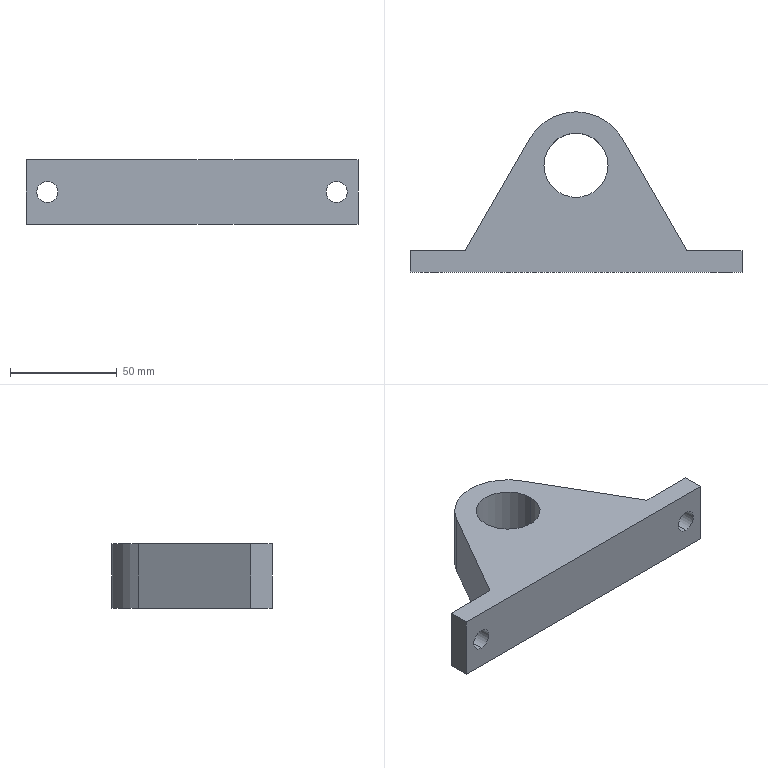Part | SolidWorks | features BaseBody 1 | 1 solid | 18 faces | box 155.5 x 75 x 30 mm | volume 151396 mm3 | plane 10 | cylinder 8 | commonest cylinder face diameters 10 x4 30 x2 50.026 x2
STEP:
#1=CARTESIAN_POINT('',(-375.282,7.138,-265.));
#2=VERTEX_POINT('',#1);
#3=CARTESIAN_POINT('',(-375.282,7.138,-275.));
#4=VERTEX_POINT('',#3);
#5=CARTESIAN_POINT('',(-375.282,7.138,-270.));
#6=DIRECTION('',(0.,-1.,0.));
#7=DIRECTION('',(0.,0.,1.));
#8=AXIS2_PLACEMENT_3D('',#5,#6,#7);
#9=CIRCLE('',#8,5.);
#10=EDGE_CURVE('',#2,#4,#9,.T.);
#11=ORIENTED_EDGE('',*,*,#10,.T.);
#12=CARTESIAN_POINT('',(-375.282,17.138,-275.));
#13=VERTEX_POINT('',#12);
#14=CARTESIAN_POINT('',(-375.282,-2.862,-275.));
#15=DIRECTION('',(0.,1.,0.));
#16=VECTOR('',#15,1000.);
#17=LINE('',#14,#16);
#18=EDGE_CURVE('',#4,#13,#17,.T.);
#19=ORIENTED_EDGE('',*,*,#18,.T.);
#20=CARTESIAN_POINT('',(-375.282,17.138,-265.));
#21=VERTEX_POINT('',#20);
#22=CARTESIAN_POINT('',(-375.282,17.138,-270.));
#23=DIRECTION('',(0.,1.,0.));
#24=DIRECTION('',(0.,0.,1.));
#25=AXIS2_PLACEMENT_3D('',#22,#23,#24);
#26=CIRCLE('',#25,5.);
#27=EDGE_CURVE('',#13,#21,#26,.T.);
#28=ORIENTED_EDGE('',*,*,#27,.T.);
#29=CARTESIAN_POINT('',(-375.282,-2.862,-265.));
#30=DIRECTION('',(0.,1.,0.));
#31=VECTOR('',#30,1000.);
#32=LINE('',#29,#31);
#33=EDGE_CURVE('',#2,#21,#32,.T.);
#34=ORIENTED_EDGE('',*,*,#33,.F.);
#35=EDGE_LOOP('',(#11,#19,#28,#34));
#36=FACE_OUTER_BOUND('',#35,.T.);
#37=CARTESIAN_POINT('',(-375.282,-2.862,-270.));
#38=DIRECTION('',(0.,1.,0.));
#39=DIRECTION('',(0.,0.,1.));
#40=AXIS2_PLACEMENT_3D('',#37,#38,#39);
#41=CYLINDRICAL_SURFACE('',#40,5.);
#42=ADVANCED_FACE('',(#36),#41,.F.);
#43=CARTESIAN_POINT('',(-510.782,7.138,-265.));
#44=VERTEX_POINT('',#43);
#45=CARTESIAN_POINT('',(-510.782,7.138,-275.));
#46=VERTEX_POINT('',#45);
#47=CARTESIAN_POINT('',(-510.782,7.138,-270.));
#48=DIRECTION('',(0.,-1.,0.));
#49=DIRECTION('',(0.,0.,1.));
#50=AXIS2_PLACEMENT_3D('',#47,#48,#49);
#51=CIRCLE('',#50,5.);
#52=EDGE_CURVE('',#44,#46,#51,.T.);
#53=ORIENTED_EDGE('',*,*,#52,.T.);
#54=CARTESIAN_POINT('',(-510.782,17.138,-275.));
#55=VERTEX_POINT('',#54);
#56=CARTESIAN_POINT('',(-510.782,-2.862,-275.));
#57=DIRECTION('',(0.,1.,0.));
#58=VECTOR('',#57,1000.);
#59=LINE('',#56,#58);
#60=EDGE_CURVE('',#46,#55,#59,.T.);
#61=ORIENTED_EDGE('',*,*,#60,.T.);
#62=CARTESIAN_POINT('',(-510.782,17.138,-265.));
#63=VERTEX_POINT('',#62);
#64=CARTESIAN_POINT('',(-510.782,17.138,-270.));
#65=DIRECTION('',(0.,1.,0.));
#66=DIRECTION('',(0.,0.,1.));
#67=AXIS2_PLACEMENT_3D('',#64,#65,#66);
#68=CIRCLE('',#67,5.);
#69=EDGE_CURVE('',#55,#63,#68,.T.);
#70=ORIENTED_EDGE('',*,*,#69,.T.);
#71=CARTESIAN_POINT('',(-510.782,-2.862,-265.));
#72=DIRECTION('',(0.,1.,0.));
#73=VECTOR('',#72,1000.);
#74=LINE('',#71,#73);
#75=EDGE_CURVE('',#44,#63,#74,.T.);
#76=ORIENTED_EDGE('',*,*,#75,.F.);
#77=EDGE_LOOP('',(#53,#61,#70,#76));
#78=FACE_OUTER_BOUND('',#77,.T.);
#79=CARTESIAN_POINT('',(-510.782,-2.862,-270.));
#80=DIRECTION('',(0.,1.,0.));
#81=DIRECTION('',(0.,0.,1.));
#82=AXIS2_PLACEMENT_3D('',#79,#80,#81);
#83=CYLINDRICAL_SURFACE('',#82,5.);
#84=ADVANCED_FACE('',(#78),#83,.F.);
#85=CARTESIAN_POINT('',(-458.032,57.138,-285.));
#86=VERTEX_POINT('',#85);
#87=CARTESIAN_POINT('',(-428.032,57.138,-285.));
#88=VERTEX_POINT('',#87);
#89=CARTESIAN_POINT('',(-443.032,57.138,-285.));
#90=DIRECTION('',(0.,0.,1.));
#91=DIRECTION('',(1.,0.,0.));
#92=AXIS2_PLACEMENT_3D('',#89,#90,#91);
#93=CIRCLE('',#92,15.);
#94=EDGE_CURVE('',#86,#88,#93,.T.);
#95=ORIENTED_EDGE('',*,*,#94,.F.);
#96=CARTESIAN_POINT('',(-458.032,57.138,-255.));
#97=VERTEX_POINT('',#96);
#98=CARTESIAN_POINT('',(-458.032,57.138,-330.));
#99=DIRECTION('',(0.,0.,1.));
#100=VECTOR('',#99,1000.);
#101=LINE('',#98,#100);
#102=EDGE_CURVE('',#86,#97,#101,.T.);
#103=ORIENTED_EDGE('',*,*,#102,.T.);
#104=CARTESIAN_POINT('',(-428.032,57.138,-255.));
#105=VERTEX_POINT('',#104);
#106=CARTESIAN_POINT('',(-443.032,57.138,-255.));
#107=DIRECTION('',(0.,0.,-1.));
#108=DIRECTION('',(-1.,0.,0.));
#109=AXIS2_PLACEMENT_3D('',#106,#107,#108);
#110=CIRCLE('',#109,15.);
#111=EDGE_CURVE('',#105,#97,#110,.T.);
#112=ORIENTED_EDGE('',*,*,#111,.F.);
#113=CARTESIAN_POINT('',(-428.032,57.138,-330.));
#114=DIRECTION('',(0.,0.,1.));
#115=VECTOR('',#114,1000.);
#116=LINE('',#113,#115);
#117=EDGE_CURVE('',#88,#105,#116,.T.);
#118=ORIENTED_EDGE('',*,*,#117,.F.);
#119=EDGE_LOOP('',(#95,#103,#112,#118));
#120=FACE_OUTER_BOUND('',#119,.T.);
#121=CARTESIAN_POINT('',(-443.032,57.138,-330.));
#122=DIRECTION('',(0.,0.,1.));
#123=DIRECTION('',(1.,0.,0.));
#124=AXIS2_PLACEMENT_3D('',#121,#122,#123);
#125=CYLINDRICAL_SURFACE('',#124,15.);
#126=ADVANCED_FACE('',(#120),#125,.F.);
#127=ORIENTED_EDGE('',*,*,#102,.F.);
#128=CARTESIAN_POINT('',(-443.032,57.138,-285.));
#129=DIRECTION('',(0.,0.,1.));
#130=DIRECTION('',(1.,0.,0.));
#131=AXIS2_PLACEMENT_3D('',#128,#129,#130);
#132=CIRCLE('',#131,15.);
#133=EDGE_CURVE('',#88,#86,#132,.T.);
#134=ORIENTED_EDGE('',*,*,#133,.F.);
#135=ORIENTED_EDGE('',*,*,#117,.T.);
#136=CARTESIAN_POINT('',(-443.032,57.138,-255.));
#137=DIRECTION('',(0.,0.,-1.));
#138=DIRECTION('',(-1.,0.,0.));
#139=AXIS2_PLACEMENT_3D('',#136,#137,#138);
#140=CIRCLE('',#139,15.);
#141=EDGE_CURVE('',#97,#105,#140,.T.);
#142=ORIENTED_EDGE('',*,*,#141,.F.);
#143=EDGE_LOOP('',(#127,#134,#135,#142));
#144=FACE_OUTER_BOUND('',#143,.T.);
#145=CARTESIAN_POINT('',(-443.032,57.138,-330.));
#146=DIRECTION('',(0.,0.,1.));
#147=DIRECTION('',(1.,0.,0.));
#148=AXIS2_PLACEMENT_3D('',#145,#146,#147);
#149=CYLINDRICAL_SURFACE('',#148,15.);
#150=ADVANCED_FACE('',(#144),#149,.F.);
#151=CARTESIAN_POINT('',(-421.37,69.645,-255.));
#152=VERTEX_POINT('',#151);
#153=CARTESIAN_POINT('',(-391.056,17.138,-255.));
#154=VERTEX_POINT('',#153);
#155=CARTESIAN_POINT('',(-446.633,113.401,-255.));
#156=DIRECTION('',(0.5,-0.866,0.));
#157=VECTOR('',#156,1000.);
#158=LINE('',#155,#157);
#159=EDGE_CURVE('',#152,#154,#158,.T.);
#160=ORIENTED_EDGE('',*,*,#159,.T.);
#161=CARTESIAN_POINT('',(-391.056,17.138,-285.));
#162=VERTEX_POINT('',#161);
#163=CARTESIAN_POINT('',(-391.056,17.138,3110.571));
#164=DIRECTION('',(0.,0.,-1.));
#165=VECTOR('',#164,1000.);
#166=LINE('',#163,#165);
#167=EDGE_CURVE('',#154,#162,#166,.T.);
#168=ORIENTED_EDGE('',*,*,#167,.T.);
#169=CARTESIAN_POINT('',(-421.37,69.645,-285.));
#170=VERTEX_POINT('',#169);
#171=CARTESIAN_POINT('',(-446.633,113.401,-285.));
#172=DIRECTION('',(-0.5,0.866,0.));
#173=VECTOR('',#172,1000.);
#174=LINE('',#171,#173);
#175=EDGE_CURVE('',#162,#170,#174,.T.);
#176=ORIENTED_EDGE('',*,*,#175,.T.);
#177=CARTESIAN_POINT('',(-421.37,69.645,3110.571));
#178=DIRECTION('',(0.,0.,-1.));
#179=VECTOR('',#178,1000.);
#180=LINE('',#177,#179);
#181=EDGE_CURVE('',#152,#170,#180,.T.);
#182=ORIENTED_EDGE('',*,*,#181,.F.);
#183=EDGE_LOOP('',(#160,#168,#176,#182));
#184=FACE_OUTER_BOUND('',#183,.T.);
#185=CARTESIAN_POINT('',(-421.37,69.645,3110.571));
#186=DIRECTION('',(0.866,0.5,0.));
#187=DIRECTION('',(-0.5,0.866,0.));
#188=AXIS2_PLACEMENT_3D('',#185,#186,#187);
#189=PLANE('',#188);
#190=ADVANCED_FACE('',(#184),#189,.T.);
#191=CARTESIAN_POINT('',(-442.227,82.138,-285.));
#192=VERTEX_POINT('',#191);
#193=CARTESIAN_POINT('',(-442.227,82.138,-255.));
#194=VERTEX_POINT('',#193);
#195=CARTESIAN_POINT('',(-442.227,82.138,3110.571));
#196=DIRECTION('',(0.,0.,1.));
#197=VECTOR('',#196,1000.);
#198=LINE('',#195,#197);
#199=EDGE_CURVE('',#192,#194,#198,.T.);
#200=ORIENTED_EDGE('',*,*,#199,.T.);
#201=CARTESIAN_POINT('',(-443.032,57.138,-255.));
#202=DIRECTION('',(0.,0.,-1.));
#203=DIRECTION('',(-1.,0.,0.));
#204=AXIS2_PLACEMENT_3D('',#201,#202,#203);
#205=CIRCLE('',#204,25.013);
#206=EDGE_CURVE('',#194,#152,#205,.T.);
#207=ORIENTED_EDGE('',*,*,#206,.T.);
#208=ORIENTED_EDGE('',*,*,#181,.T.);
#209=CARTESIAN_POINT('',(-443.032,57.138,-285.));
#210=DIRECTION('',(0.,0.,1.));
#211=DIRECTION('',(1.,0.,0.));
#212=AXIS2_PLACEMENT_3D('',#209,#210,#211);
#213=CIRCLE('',#212,25.013);
#214=EDGE_CURVE('',#170,#192,#213,.T.);
#215=ORIENTED_EDGE('',*,*,#214,.T.);
#216=EDGE_LOOP('',(#200,#207,#208,#215));
#217=FACE_OUTER_BOUND('',#216,.T.);
#218=CARTESIAN_POINT('',(-443.032,57.138,3110.571));
#219=DIRECTION('',(0.,0.,-1.));
#220=DIRECTION('',(-1.,0.,0.));
#221=AXIS2_PLACEMENT_3D('',#218,#219,#220);
#222=CYLINDRICAL_SURFACE('',#221,25.013);
#223=ADVANCED_FACE('',(#217),#222,.T.);
#224=CARTESIAN_POINT('',(-443.838,82.138,-255.));
#225=VERTEX_POINT('',#224);
#226=CARTESIAN_POINT('',(-443.838,82.138,-285.));
#227=VERTEX_POINT('',#226);
#228=CARTESIAN_POINT('',(-443.838,82.138,3110.571));
#229=DIRECTION('',(0.,0.,-1.));
#230=VECTOR('',#229,1000.);
#231=LINE('',#228,#230);
#232=EDGE_CURVE('',#225,#227,#231,.T.);
#233=ORIENTED_EDGE('',*,*,#232,.F.);
#234=CARTESIAN_POINT('',(-616.782,82.138,-255.));
#235=DIRECTION('',(1.,0.,0.));
#236=VECTOR('',#235,1000.);
#237=LINE('',#234,#236);
#238=EDGE_CURVE('',#225,#194,#237,.T.);
#239=ORIENTED_EDGE('',*,*,#238,.T.);
#240=ORIENTED_EDGE('',*,*,#199,.F.);
#241=CARTESIAN_POINT('',(-616.782,82.138,-285.));
#242=DIRECTION('',(-1.,0.,0.));
#243=VECTOR('',#242,1000.);
#244=LINE('',#241,#243);
#245=EDGE_CURVE('',#192,#227,#244,.T.);
#246=ORIENTED_EDGE('',*,*,#245,.T.);
#247=EDGE_LOOP('',(#233,#239,#240,#246));
#248=FACE_OUTER_BOUND('',#247,.T.);
#249=CARTESIAN_POINT('',(-616.782,82.138,70.));
#250=DIRECTION('',(0.,-1.,0.));
#251=DIRECTION('',(0.,0.,-1.));
#252=AXIS2_PLACEMENT_3D('',#249,#250,#251);
#253=PLANE('',#252);
#254=ADVANCED_FACE('',(#248),#253,.F.);
#255=CARTESIAN_POINT('',(-464.694,69.645,-255.));
#256=VERTEX_POINT('',#255);
#257=CARTESIAN_POINT('',(-464.694,69.645,-285.));
#258=VERTEX_POINT('',#257);
#259=CARTESIAN_POINT('',(-464.694,69.645,3110.571));
#260=DIRECTION('',(0.,0.,-1.));
#261=VECTOR('',#260,1000.);
#262=LINE('',#259,#261);
#263=EDGE_CURVE('',#256,#258,#262,.T.);
#264=ORIENTED_EDGE('',*,*,#263,.F.);
#265=CARTESIAN_POINT('',(-443.032,57.138,-255.));
#266=DIRECTION('',(0.,0.,-1.));
#267=DIRECTION('',(-1.,0.,0.));
#268=AXIS2_PLACEMENT_3D('',#265,#266,#267);
#269=CIRCLE('',#268,25.013);
#270=EDGE_CURVE('',#256,#225,#269,.T.);
#271=ORIENTED_EDGE('',*,*,#270,.T.);
#272=ORIENTED_EDGE('',*,*,#232,.T.);
#273=CARTESIAN_POINT('',(-443.032,57.138,-285.));
#274=DIRECTION('',(0.,0.,1.));
#275=DIRECTION('',(1.,0.,0.));
#276=AXIS2_PLACEMENT_3D('',#273,#274,#275);
#277=CIRCLE('',#276,25.013);
#278=EDGE_CURVE('',#227,#258,#277,.T.);
#279=ORIENTED_EDGE('',*,*,#278,.T.);
#280=EDGE_LOOP('',(#264,#271,#272,#279));
#281=FACE_OUTER_BOUND('',#280,.T.);
#282=CARTESIAN_POINT('',(-443.032,57.138,3110.571));
#283=DIRECTION('',(0.,0.,-1.));
#284=DIRECTION('',(-1.,0.,0.));
#285=AXIS2_PLACEMENT_3D('',#282,#283,#284);
#286=CYLINDRICAL_SURFACE('',#285,25.013);
#287=ADVANCED_FACE('',(#281),#286,.T.);
#288=CARTESIAN_POINT('',(-495.009,17.138,-255.));
#289=VERTEX_POINT('',#288);
#290=CARTESIAN_POINT('',(-495.009,17.138,-285.));
#291=VERTEX_POINT('',#290);
#292=CARTESIAN_POINT('',(-495.009,17.138,3110.571));
#293=DIRECTION('',(0.,0.,-1.));
#294=VECTOR('',#293,1000.);
#295=LINE('',#292,#294);
#296=EDGE_CURVE('',#289,#291,#295,.T.);
#297=ORIENTED_EDGE('',*,*,#296,.F.);
#298=CARTESIAN_POINT('',(-468.306,63.388,-255.));
#299=DIRECTION('',(0.5,0.866,0.));
#300=VECTOR('',#299,1000.);
#301=LINE('',#298,#300);
#302=EDGE_CURVE('',#289,#256,#301,.T.);
#303=ORIENTED_EDGE('',*,*,#302,.T.);
#304=ORIENTED_EDGE('',*,*,#263,.T.);
#305=CARTESIAN_POINT('',(-468.306,63.388,-285.));
#306=DIRECTION('',(-0.5,-0.866,0.));
#307=VECTOR('',#306,1000.);
#308=LINE('',#305,#307);
#309=EDGE_CURVE('',#258,#291,#308,.T.);
#310=ORIENTED_EDGE('',*,*,#309,.T.);
#311=EDGE_LOOP('',(#297,#303,#304,#310));
#312=FACE_OUTER_BOUND('',#311,.T.);
#313=CARTESIAN_POINT('',(-464.694,69.645,3110.571));
#314=DIRECTION('',(-0.866,0.5,0.));
#315=DIRECTION('',(-0.5,-0.866,0.));
#316=AXIS2_PLACEMENT_3D('',#313,#314,#315);
#317=PLANE('',#316);
#318=ADVANCED_FACE('',(#312),#317,.T.);
#319=CARTESIAN_POINT('',(-365.282,7.138,-255.));
#320=VERTEX_POINT('',#319);
#321=CARTESIAN_POINT('',(-365.282,7.138,-285.));
#322=VERTEX_POINT('',#321);
#323=CARTESIAN_POINT('',(-365.282,7.138,-280.));
#324=DIRECTION('',(0.,0.,-1.));
#325=VECTOR('',#324,1000.);
#326=LINE('',#323,#325);
#327=EDGE_CURVE('',#320,#322,#326,.T.);
#328=ORIENTED_EDGE('',*,*,#327,.T.);
#329=CARTESIAN_POINT('',(-365.282,17.138,-285.));
#330=VERTEX_POINT('',#329);
#331=CARTESIAN_POINT('',(-365.282,82.138,-285.));
#332=DIRECTION('',(0.,-1.,0.));
#333=VECTOR('',#332,1000.);
#334=LINE('',#331,#333);
#335=EDGE_CURVE('',#330,#322,#334,.T.);
#336=ORIENTED_EDGE('',*,*,#335,.F.);
#337=CARTESIAN_POINT('',(-365.282,17.138,-255.));
#338=VERTEX_POINT('',#337);
#339=CARTESIAN_POINT('',(-365.282,17.138,-280.));
#340=DIRECTION('',(0.,0.,-1.));
#341=VECTOR('',#340,1000.);
#342=LINE('',#339,#341);
#343=EDGE_CURVE('',#338,#330,#342,.T.);
#344=ORIENTED_EDGE('',*,*,#343,.F.);
#345=CARTESIAN_POINT('',(-365.282,17.138,-255.));
#346=DIRECTION('',(0.,-1.,0.));
#347=VECTOR('',#346,1000.);
#348=LINE('',#345,#347);
#349=EDGE_CURVE('',#338,#320,#348,.T.);
#350=ORIENTED_EDGE('',*,*,#349,.T.);
#351=EDGE_LOOP('',(#328,#336,#344,#350));
#352=FACE_OUTER_BOUND('',#351,.T.);
#353=CARTESIAN_POINT('',(-365.282,17.138,-280.));
#354=DIRECTION('',(-1.,0.,0.));
#355=DIRECTION('',(0.,0.,1.));
#356=AXIS2_PLACEMENT_3D('',#353,#354,#355);
#357=PLANE('',#356);
#358=ADVANCED_FACE('',(#352),#357,.F.);
#359=CARTESIAN_POINT('',(-520.782,7.138,-285.));
#360=VERTEX_POINT('',#359);
#361=CARTESIAN_POINT('',(-520.782,7.138,-255.));
#362=VERTEX_POINT('',#361);
#363=CARTESIAN_POINT('',(-520.782,7.138,-280.));
#364=DIRECTION('',(0.,0.,1.));
#365=VECTOR('',#364,1000.);
#366=LINE('',#363,#365);
#367=EDGE_CURVE('',#360,#362,#366,.T.);
#368=ORIENTED_EDGE('',*,*,#367,.T.);
#369=CARTESIAN_POINT('',(-520.782,17.138,-255.));
#370=VERTEX_POINT('',#369);
#371=CARTESIAN_POINT('',(-520.782,82.138,-255.));
#372=DIRECTION('',(0.,-1.,0.));
#373=VECTOR('',#372,1000.);
#374=LINE('',#371,#373);
#375=EDGE_CURVE('',#370,#362,#374,.T.);
#376=ORIENTED_EDGE('',*,*,#375,.F.);
#377=CARTESIAN_POINT('',(-520.782,17.138,-285.));
#378=VERTEX_POINT('',#377);
#379=CARTESIAN_POINT('',(-520.782,17.138,-280.));
#380=DIRECTION('',(0.,0.,1.));
#381=VECTOR('',#380,1000.);
#382=LINE('',#379,#381);
#383=EDGE_CURVE('',#378,#370,#382,.T.);
#384=ORIENTED_EDGE('',*,*,#383,.F.);
#385=CARTESIAN_POINT('',(-520.782,17.138,-285.));
#386=DIRECTION('',(0.,-1.,0.));
#387=VECTOR('',#386,1000.);
#388=LINE('',#385,#387);
#389=EDGE_CURVE('',#378,#360,#388,.T.);
#390=ORIENTED_EDGE('',*,*,#389,.T.);
#391=EDGE_LOOP('',(#368,#376,#384,#390));
#392=FACE_OUTER_BOUND('',#391,.T.);
#393=CARTESIAN_POINT('',(-520.782,17.138,-280.));
#394=DIRECTION('',(1.,0.,0.));
#395=DIRECTION('',(0.,0.,-1.));
#396=AXIS2_PLACEMENT_3D('',#393,#394,#395);
#397=PLANE('',#396);
#398=ADVANCED_FACE('',(#392),#397,.F.);
#399=CARTESIAN_POINT('',(-500.782,7.138,-285.));
#400=DIRECTION('',(-1.,0.,0.));
#401=VECTOR('',#400,1000.);
#402=LINE('',#399,#401);
#403=EDGE_CURVE('',#322,#360,#402,.T.);
#404=ORIENTED_EDGE('',*,*,#403,.T.);
#405=ORIENTED_EDGE('',*,*,#389,.F.);
#406=CARTESIAN_POINT('',(-500.782,17.138,-285.));
#407=DIRECTION('',(-1.,0.,0.));
#408=VECTOR('',#407,1000.);
#409=LINE('',#406,#408);
#410=EDGE_CURVE('',#291,#378,#409,.T.);
#411=ORIENTED_EDGE('',*,*,#410,.F.);
#412=ORIENTED_EDGE('',*,*,#309,.F.);
#413=ORIENTED_EDGE('',*,*,#278,.F.);
#414=ORIENTED_EDGE('',*,*,#245,.F.);
#415=ORIENTED_EDGE('',*,*,#214,.F.);
#416=ORIENTED_EDGE('',*,*,#175,.F.);
#417=CARTESIAN_POINT('',(-616.782,17.138,-285.));
#418=DIRECTION('',(-1.,0.,0.));
#419=VECTOR('',#418,1000.);
#420=LINE('',#417,#419);
#421=EDGE_CURVE('',#330,#162,#420,.T.);
#422=ORIENTED_EDGE('',*,*,#421,.F.);
#423=ORIENTED_EDGE('',*,*,#335,.T.);
#424=EDGE_LOOP('',(#404,#405,#411,#412,#413,#414,#415,#416,#422,#423));
#425=FACE_OUTER_BOUND('',#424,.T.);
#426=ORIENTED_EDGE('',*,*,#133,.T.);
#427=ORIENTED_EDGE('',*,*,#94,.T.);
#428=EDGE_LOOP('',(#426,#427));
#429=FACE_BOUND('',#428,.T.);
#430=CARTESIAN_POINT('',(-500.782,82.138,-285.));
#431=DIRECTION('',(0.,0.,1.));
#432=DIRECTION('',(1.,0.,0.));
#433=AXIS2_PLACEMENT_3D('',#430,#431,#432);
#434=PLANE('',#433);
#435=ADVANCED_FACE('',(#425,#429),#434,.F.);
#436=CARTESIAN_POINT('',(-500.782,7.138,-255.));
#437=DIRECTION('',(1.,0.,0.));
#438=VECTOR('',#437,1000.);
#439=LINE('',#436,#438);
#440=EDGE_CURVE('',#362,#320,#439,.T.);
#441=ORIENTED_EDGE('',*,*,#440,.T.);
#442=ORIENTED_EDGE('',*,*,#349,.F.);
#443=CARTESIAN_POINT('',(-616.782,17.138,-255.));
#444=DIRECTION('',(1.,0.,0.));
#445=VECTOR('',#444,1000.);
#446=LINE('',#443,#445);
#447=EDGE_CURVE('',#154,#338,#446,.T.);
#448=ORIENTED_EDGE('',*,*,#447,.F.);
#449=ORIENTED_EDGE('',*,*,#159,.F.);
#450=ORIENTED_EDGE('',*,*,#206,.F.);
#451=ORIENTED_EDGE('',*,*,#238,.F.);
#452=ORIENTED_EDGE('',*,*,#270,.F.);
#453=ORIENTED_EDGE('',*,*,#302,.F.);
#454=CARTESIAN_POINT('',(-500.782,17.138,-255.));
#455=DIRECTION('',(1.,0.,0.));
#456=VECTOR('',#455,1000.);
#457=LINE('',#454,#456);
#458=EDGE_CURVE('',#370,#289,#457,.T.);
#459=ORIENTED_EDGE('',*,*,#458,.F.);
#460=ORIENTED_EDGE('',*,*,#375,.T.);
#461=EDGE_LOOP('',(#441,#442,#448,#449,#450,#451,#452,#453,#459,#460));
#462=FACE_OUTER_BOUND('',#461,.T.);
#463=ORIENTED_EDGE('',*,*,#111,.T.);
#464=ORIENTED_EDGE('',*,*,#141,.T.);
#465=EDGE_LOOP('',(#463,#464));
#466=FACE_BOUND('',#465,.T.);
#467=CARTESIAN_POINT('',(-500.782,82.138,-255.));
#468=DIRECTION('',(0.,0.,-1.));
#469=DIRECTION('',(-1.,0.,0.));
#470=AXIS2_PLACEMENT_3D('',#467,#468,#469);
#471=PLANE('',#470);
#472=ADVANCED_FACE('',(#462,#466),#471,.F.);
#473=CARTESIAN_POINT('',(-510.782,17.138,-270.));
#474=DIRECTION('',(0.,1.,0.));
#475=DIRECTION('',(0.,0.,1.));
#476=AXIS2_PLACEMENT_3D('',#473,#474,#475);
#477=CIRCLE('',#476,5.);
#478=EDGE_CURVE('',#63,#55,#477,.T.);
#479=ORIENTED_EDGE('',*,*,#478,.F.);
#480=ORIENTED_EDGE('',*,*,#69,.F.);
#481=EDGE_LOOP('',(#479,#480));
#482=FACE_BOUND('',#481,.T.);
#483=ORIENTED_EDGE('',*,*,#458,.T.);
#484=ORIENTED_EDGE('',*,*,#296,.T.);
#485=ORIENTED_EDGE('',*,*,#410,.T.);
#486=ORIENTED_EDGE('',*,*,#383,.T.);
#487=EDGE_LOOP('',(#483,#484,#485,#486));
#488=FACE_OUTER_BOUND('',#487,.T.);
#489=CARTESIAN_POINT('',(-616.782,17.138,70.));
#490=DIRECTION('',(0.,1.,0.));
#491=DIRECTION('',(0.,0.,1.));
#492=AXIS2_PLACEMENT_3D('',#489,#490,#491);
#493=PLANE('',#492);
#494=ADVANCED_FACE('',(#482,#488),#493,.T.);
#495=ORIENTED_EDGE('',*,*,#60,.F.);
#496=CARTESIAN_POINT('',(-510.782,7.138,-270.));
#497=DIRECTION('',(0.,-1.,0.));
#498=DIRECTION('',(0.,0.,1.));
#499=AXIS2_PLACEMENT_3D('',#496,#497,#498);
#500=CIRCLE('',#499,5.);
#501=EDGE_CURVE('',#46,#44,#500,.T.);
#502=ORIENTED_EDGE('',*,*,#501,.T.);
#503=ORIENTED_EDGE('',*,*,#75,.T.);
#504=ORIENTED_EDGE('',*,*,#478,.T.);
#505=EDGE_LOOP('',(#495,#502,#503,#504));
#506=FACE_OUTER_BOUND('',#505,.T.);
#507=CARTESIAN_POINT('',(-510.782,-2.862,-270.));
#508=DIRECTION('',(0.,1.,0.));
#509=DIRECTION('',(0.,0.,1.));
#510=AXIS2_PLACEMENT_3D('',#507,#508,#509);
#511=CYLINDRICAL_SURFACE('',#510,5.);
#512=ADVANCED_FACE('',(#506),#511,.F.);
#513=CARTESIAN_POINT('',(-375.282,17.138,-270.));
#514=DIRECTION('',(0.,1.,0.));
#515=DIRECTION('',(0.,0.,1.));
#516=AXIS2_PLACEMENT_3D('',#513,#514,#515);
#517=CIRCLE('',#516,5.);
#518=EDGE_CURVE('',#21,#13,#517,.T.);
#519=ORIENTED_EDGE('',*,*,#518,.F.);
#520=ORIENTED_EDGE('',*,*,#27,.F.);
#521=EDGE_LOOP('',(#519,#520));
#522=FACE_BOUND('',#521,.T.);
#523=ORIENTED_EDGE('',*,*,#167,.F.);
#524=ORIENTED_EDGE('',*,*,#447,.T.);
#525=ORIENTED_EDGE('',*,*,#343,.T.);
#526=ORIENTED_EDGE('',*,*,#421,.T.);
#527=EDGE_LOOP('',(#523,#524,#525,#526));
#528=FACE_OUTER_BOUND('',#527,.T.);
#529=CARTESIAN_POINT('',(-616.782,17.138,70.));
#530=DIRECTION('',(0.,-1.,0.));
#531=DIRECTION('',(0.,0.,-1.));
#532=AXIS2_PLACEMENT_3D('',#529,#530,#531);
#533=PLANE('',#532);
#534=ADVANCED_FACE('',(#522,#528),#533,.F.);
#535=ORIENTED_EDGE('',*,*,#18,.F.);
#536=CARTESIAN_POINT('',(-375.282,7.138,-270.));
#537=DIRECTION('',(0.,-1.,0.));
#538=DIRECTION('',(0.,0.,1.));
#539=AXIS2_PLACEMENT_3D('',#536,#537,#538);
#540=CIRCLE('',#539,5.);
#541=EDGE_CURVE('',#4,#2,#540,.T.);
#542=ORIENTED_EDGE('',*,*,#541,.T.);
#543=ORIENTED_EDGE('',*,*,#33,.T.);
#544=ORIENTED_EDGE('',*,*,#518,.T.);
#545=EDGE_LOOP('',(#535,#542,#543,#544));
#546=FACE_OUTER_BOUND('',#545,.T.);
#547=CARTESIAN_POINT('',(-375.282,-2.862,-270.));
#548=DIRECTION('',(0.,1.,0.));
#549=DIRECTION('',(0.,0.,1.));
#550=AXIS2_PLACEMENT_3D('',#547,#548,#549);
#551=CYLINDRICAL_SURFACE('',#550,5.);
#552=ADVANCED_FACE('',(#546),#551,.F.);
#553=ORIENTED_EDGE('',*,*,#10,.F.);
#554=ORIENTED_EDGE('',*,*,#541,.F.);
#555=EDGE_LOOP('',(#553,#554));
#556=FACE_BOUND('',#555,.T.);
#557=ORIENTED_EDGE('',*,*,#52,.F.);
#558=ORIENTED_EDGE('',*,*,#501,.F.);
#559=EDGE_LOOP('',(#557,#558));
#560=FACE_BOUND('',#559,.T.);
#561=ORIENTED_EDGE('',*,*,#440,.F.);
#562=ORIENTED_EDGE('',*,*,#367,.F.);
#563=ORIENTED_EDGE('',*,*,#403,.F.);
#564=ORIENTED_EDGE('',*,*,#327,.F.);
#565=EDGE_LOOP('',(#561,#562,#563,#564));
#566=FACE_OUTER_BOUND('',#565,.T.);
#567=CARTESIAN_POINT('',(-41.782,7.138,70.));
#568=DIRECTION('',(0.,1.,0.));
#569=DIRECTION('',(0.,0.,1.));
#570=AXIS2_PLACEMENT_3D('',#567,#568,#569);
#571=PLANE('',#570);
#572=ADVANCED_FACE('',(#556,#560,#566),#571,.F.);
#573=CLOSED_SHELL('',(#42,#84,#126,#150,#190,#223,#254,#287,#318,#358,#398,#435,#472,#494,#512,#534,#552,#572));
#574=MANIFOLD_SOLID_BREP('',#573);
#575=CARTESIAN_POINT('',(0.,0.,0.));
#576=DIRECTION('',(0.,0.,1.));
#577=DIRECTION('',(1.,0.,0.));
#578=AXIS2_PLACEMENT_3D('',#575,#576,#577);
#579=(LENGTH_UNIT()NAMED_UNIT(*)SI_UNIT(.MILLI.,.METRE.));
#580=UNCERTAINTY_MEASURE_WITH_UNIT(LENGTH_MEASURE(0.00001),#579,'','');
#581=(NAMED_UNIT(*)PLANE_ANGLE_UNIT()SI_UNIT($,.RADIAN.));
#582=(NAMED_UNIT(*)SI_UNIT($,.STERADIAN.)SOLID_ANGLE_UNIT());
#583=(GEOMETRIC_REPRESENTATION_CONTEXT(3)GLOBAL_UNCERTAINTY_ASSIGNED_CONTEXT((#580))GLOBAL_UNIT_ASSIGNED_CONTEXT((#579,#581,#582))REPRESENTATION_CONTEXT('',''));
#584=ADVANCED_BREP_SHAPE_REPRESENTATION('',(#574,#578),#583);